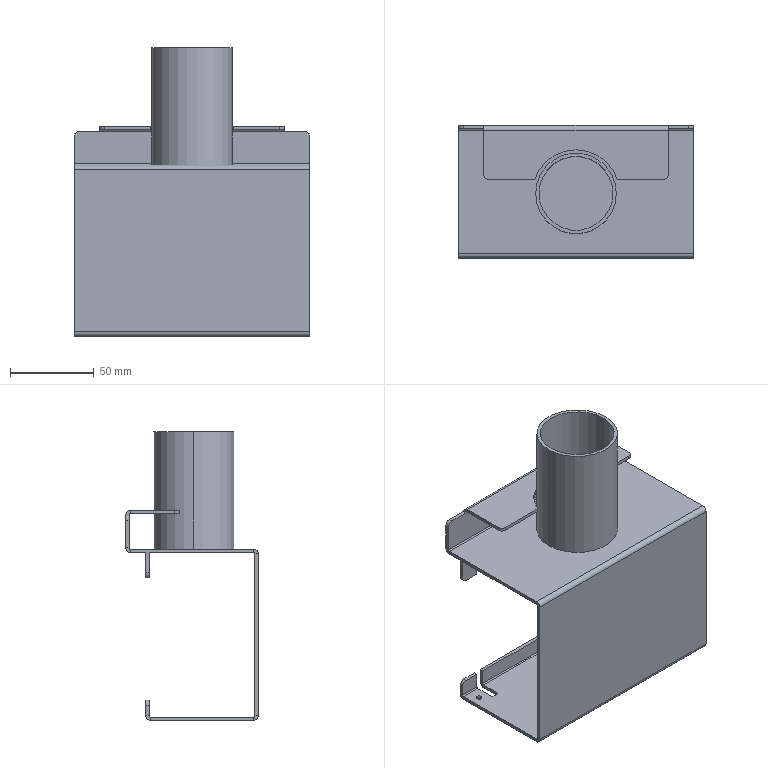Part | STEP file | H_ND25042-01-JG-003B-BJ | 1 solid | 110 faces | box 140 x 79 x 172 mm | volume 102323 mm3 | plane 71 | cylinder 39 | commonest cylinder face diameters 1 x8 6 x8 1.473 x7 5.473 x7 3.3 x4 44 x2